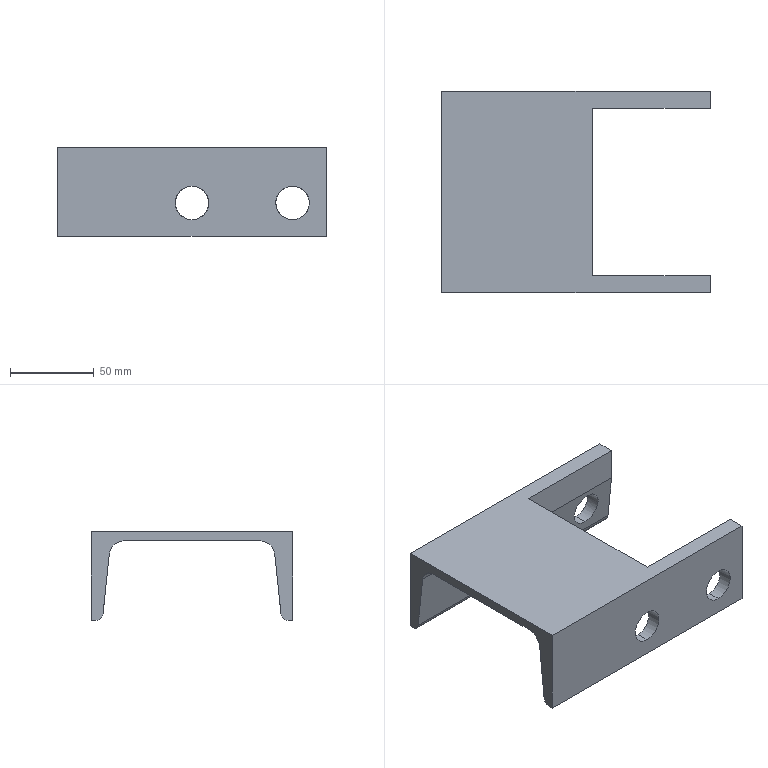Part | SolidWorks | features ICE 2, 3DProfileFeature 1, WeldMemberFeat 1, WeldmentFeature 1 | 1 solid | 26 faces | box 160 x 120 x 53 mm | volume 192954 mm3 | plane 14 | cylinder 12 | commonest cylinder face diameters 20 x8 9 x2 18 x2
STEP:
#1=CARTESIAN_POINT('',(80.,9.657,-23.));
#2=VERTEX_POINT('',#1);
#3=CARTESIAN_POINT('',(80.,7.555,-43.));
#4=VERTEX_POINT('',#3);
#5=CARTESIAN_POINT('',(80.,9.657,-23.));
#6=CARTESIAN_POINT('',(60.,9.657,-23.));
#7=CARTESIAN_POINT('',(60.,7.555,-43.));
#8=CARTESIAN_POINT('',(80.,7.555,-43.));
#9=(BOUNDED_CURVE()B_SPLINE_CURVE(3,(#5,#6,#7,#8),.UNSPECIFIED.,.F.,.F.)B_SPLINE_CURVE_WITH_KNOTS((4,4),(3.142,6.283),.UNSPECIFIED.)CURVE()GEOMETRIC_REPRESENTATION_ITEM()RATIONAL_B_SPLINE_CURVE((1.,0.3333,0.3333,1.))REPRESENTATION_ITEM(''));
#10=EDGE_CURVE('',#2,#4,#9,.T.);
#11=ORIENTED_EDGE('',*,*,#10,.F.);
#12=CARTESIAN_POINT('',(80.,0.,-23.));
#13=VERTEX_POINT('',#12);
#14=CARTESIAN_POINT('',(80.,148.284,-23.));
#15=DIRECTION('',(0.,-1.,0.));
#16=VECTOR('',#15,1000.);
#17=LINE('',#14,#16);
#18=EDGE_CURVE('',#2,#13,#17,.T.);
#19=ORIENTED_EDGE('',*,*,#18,.T.);
#20=CARTESIAN_POINT('',(80.,0.,-43.));
#21=VERTEX_POINT('',#20);
#22=CARTESIAN_POINT('',(80.,0.,-33.));
#23=DIRECTION('',(0.,-1.,0.));
#24=DIRECTION('',(0.,0.,-1.));
#25=AXIS2_PLACEMENT_3D('',#22,#23,#24);
#26=CIRCLE('',#25,10.);
#27=EDGE_CURVE('',#13,#21,#26,.T.);
#28=ORIENTED_EDGE('',*,*,#27,.T.);
#29=CARTESIAN_POINT('',(80.,148.284,-43.));
#30=DIRECTION('',(0.,-1.,0.));
#31=VECTOR('',#30,1000.);
#32=LINE('',#29,#31);
#33=EDGE_CURVE('',#4,#21,#32,.T.);
#34=ORIENTED_EDGE('',*,*,#33,.F.);
#35=EDGE_LOOP('',(#11,#19,#28,#34));
#36=FACE_OUTER_BOUND('',#35,.T.);
#37=CARTESIAN_POINT('',(80.,148.284,-33.));
#38=DIRECTION('',(0.,-1.,0.));
#39=DIRECTION('',(0.,0.,-1.));
#40=AXIS2_PLACEMENT_3D('',#37,#38,#39);
#41=CYLINDRICAL_SURFACE('',#40,10.);
#42=ADVANCED_FACE('',(#36),#41,.F.);
#43=CARTESIAN_POINT('',(80.,120.,-43.));
#44=VERTEX_POINT('',#43);
#45=CARTESIAN_POINT('',(80.,120.,-23.));
#46=VERTEX_POINT('',#45);
#47=CARTESIAN_POINT('',(80.,120.,-33.));
#48=DIRECTION('',(0.,1.,0.));
#49=DIRECTION('',(0.,0.,-1.));
#50=AXIS2_PLACEMENT_3D('',#47,#48,#49);
#51=CIRCLE('',#50,10.);
#52=EDGE_CURVE('',#44,#46,#51,.T.);
#53=ORIENTED_EDGE('',*,*,#52,.T.);
#54=CARTESIAN_POINT('',(80.,110.343,-23.));
#55=VERTEX_POINT('',#54);
#56=CARTESIAN_POINT('',(80.,148.284,-23.));
#57=DIRECTION('',(0.,-1.,0.));
#58=VECTOR('',#57,1000.);
#59=LINE('',#56,#58);
#60=EDGE_CURVE('',#46,#55,#59,.T.);
#61=ORIENTED_EDGE('',*,*,#60,.T.);
#62=CARTESIAN_POINT('',(80.,112.445,-43.));
#63=VERTEX_POINT('',#62);
#64=CARTESIAN_POINT('',(80.,112.445,-43.));
#65=CARTESIAN_POINT('',(60.,112.445,-43.));
#66=CARTESIAN_POINT('',(60.,110.343,-23.));
#67=CARTESIAN_POINT('',(80.,110.343,-23.));
#68=(BOUNDED_CURVE()B_SPLINE_CURVE(3,(#64,#65,#66,#67),.UNSPECIFIED.,.F.,.F.)B_SPLINE_CURVE_WITH_KNOTS((4,4),(3.142,6.283),.UNSPECIFIED.)CURVE()GEOMETRIC_REPRESENTATION_ITEM()RATIONAL_B_SPLINE_CURVE((1.,0.3333,0.3333,1.))REPRESENTATION_ITEM(''));
#69=EDGE_CURVE('',#63,#55,#68,.T.);
#70=ORIENTED_EDGE('',*,*,#69,.F.);
#71=CARTESIAN_POINT('',(80.,148.284,-43.));
#72=DIRECTION('',(0.,-1.,0.));
#73=VECTOR('',#72,1000.);
#74=LINE('',#71,#73);
#75=EDGE_CURVE('',#44,#63,#74,.T.);
#76=ORIENTED_EDGE('',*,*,#75,.F.);
#77=EDGE_LOOP('',(#53,#61,#70,#76));
#78=FACE_OUTER_BOUND('',#77,.T.);
#79=CARTESIAN_POINT('',(80.,148.284,-33.));
#80=DIRECTION('',(0.,-1.,0.));
#81=DIRECTION('',(0.,0.,-1.));
#82=AXIS2_PLACEMENT_3D('',#79,#80,#81);
#83=CYLINDRICAL_SURFACE('',#82,10.);
#84=ADVANCED_FACE('',(#78),#83,.F.);
#85=CARTESIAN_POINT('',(140.,9.657,-23.));
#86=VERTEX_POINT('',#85);
#87=CARTESIAN_POINT('',(140.,7.555,-43.));
#88=VERTEX_POINT('',#87);
#89=CARTESIAN_POINT('',(140.,9.657,-23.));
#90=CARTESIAN_POINT('',(120.,9.657,-23.));
#91=CARTESIAN_POINT('',(120.,7.555,-43.));
#92=CARTESIAN_POINT('',(140.,7.555,-43.));
#93=(BOUNDED_CURVE()B_SPLINE_CURVE(3,(#89,#90,#91,#92),.UNSPECIFIED.,.F.,.F.)B_SPLINE_CURVE_WITH_KNOTS((4,4),(3.142,6.283),.UNSPECIFIED.)CURVE()GEOMETRIC_REPRESENTATION_ITEM()RATIONAL_B_SPLINE_CURVE((1.,0.3333,0.3333,1.))REPRESENTATION_ITEM(''));
#94=EDGE_CURVE('',#86,#88,#93,.T.);
#95=ORIENTED_EDGE('',*,*,#94,.F.);
#96=CARTESIAN_POINT('',(140.,0.,-23.));
#97=VERTEX_POINT('',#96);
#98=CARTESIAN_POINT('',(140.,148.284,-23.));
#99=DIRECTION('',(0.,-1.,0.));
#100=VECTOR('',#99,1000.);
#101=LINE('',#98,#100);
#102=EDGE_CURVE('',#86,#97,#101,.T.);
#103=ORIENTED_EDGE('',*,*,#102,.T.);
#104=CARTESIAN_POINT('',(140.,0.,-43.));
#105=VERTEX_POINT('',#104);
#106=CARTESIAN_POINT('',(140.,0.,-33.));
#107=DIRECTION('',(0.,-1.,0.));
#108=DIRECTION('',(0.,0.,-1.));
#109=AXIS2_PLACEMENT_3D('',#106,#107,#108);
#110=CIRCLE('',#109,10.);
#111=EDGE_CURVE('',#97,#105,#110,.T.);
#112=ORIENTED_EDGE('',*,*,#111,.T.);
#113=CARTESIAN_POINT('',(140.,148.284,-43.));
#114=DIRECTION('',(0.,-1.,0.));
#115=VECTOR('',#114,1000.);
#116=LINE('',#113,#115);
#117=EDGE_CURVE('',#88,#105,#116,.T.);
#118=ORIENTED_EDGE('',*,*,#117,.F.);
#119=EDGE_LOOP('',(#95,#103,#112,#118));
#120=FACE_OUTER_BOUND('',#119,.T.);
#121=CARTESIAN_POINT('',(140.,148.284,-33.));
#122=DIRECTION('',(0.,-1.,0.));
#123=DIRECTION('',(0.,0.,-1.));
#124=AXIS2_PLACEMENT_3D('',#121,#122,#123);
#125=CYLINDRICAL_SURFACE('',#124,10.);
#126=ADVANCED_FACE('',(#120),#125,.F.);
#127=CARTESIAN_POINT('',(140.,120.,-43.));
#128=VERTEX_POINT('',#127);
#129=CARTESIAN_POINT('',(140.,120.,-23.));
#130=VERTEX_POINT('',#129);
#131=CARTESIAN_POINT('',(140.,120.,-33.));
#132=DIRECTION('',(0.,1.,0.));
#133=DIRECTION('',(0.,0.,-1.));
#134=AXIS2_PLACEMENT_3D('',#131,#132,#133);
#135=CIRCLE('',#134,10.);
#136=EDGE_CURVE('',#128,#130,#135,.T.);
#137=ORIENTED_EDGE('',*,*,#136,.T.);
#138=CARTESIAN_POINT('',(140.,110.343,-23.));
#139=VERTEX_POINT('',#138);
#140=CARTESIAN_POINT('',(140.,148.284,-23.));
#141=DIRECTION('',(0.,-1.,0.));
#142=VECTOR('',#141,1000.);
#143=LINE('',#140,#142);
#144=EDGE_CURVE('',#130,#139,#143,.T.);
#145=ORIENTED_EDGE('',*,*,#144,.T.);
#146=CARTESIAN_POINT('',(140.,112.445,-43.));
#147=VERTEX_POINT('',#146);
#148=CARTESIAN_POINT('',(140.,112.445,-43.));
#149=CARTESIAN_POINT('',(120.,112.445,-43.));
#150=CARTESIAN_POINT('',(120.,110.343,-23.));
#151=CARTESIAN_POINT('',(140.,110.343,-23.));
#152=(BOUNDED_CURVE()B_SPLINE_CURVE(3,(#148,#149,#150,#151),.UNSPECIFIED.,.F.,.F.)B_SPLINE_CURVE_WITH_KNOTS((4,4),(3.142,6.283),.UNSPECIFIED.)CURVE()GEOMETRIC_REPRESENTATION_ITEM()RATIONAL_B_SPLINE_CURVE((1.,0.3333,0.3333,1.))REPRESENTATION_ITEM(''));
#153=EDGE_CURVE('',#147,#139,#152,.T.);
#154=ORIENTED_EDGE('',*,*,#153,.F.);
#155=CARTESIAN_POINT('',(140.,148.284,-43.));
#156=DIRECTION('',(0.,-1.,0.));
#157=VECTOR('',#156,1000.);
#158=LINE('',#155,#157);
#159=EDGE_CURVE('',#128,#147,#158,.T.);
#160=ORIENTED_EDGE('',*,*,#159,.F.);
#161=EDGE_LOOP('',(#137,#145,#154,#160));
#162=FACE_OUTER_BOUND('',#161,.T.);
#163=CARTESIAN_POINT('',(140.,148.284,-33.));
#164=DIRECTION('',(0.,-1.,0.));
#165=DIRECTION('',(0.,0.,-1.));
#166=AXIS2_PLACEMENT_3D('',#163,#164,#165);
#167=CYLINDRICAL_SURFACE('',#166,10.);
#168=ADVANCED_FACE('',(#162),#167,.F.);
#169=CARTESIAN_POINT('',(160.,110.,-19.736));
#170=VERTEX_POINT('',#169);
#171=CARTESIAN_POINT('',(160.,110.,0.));
#172=VERTEX_POINT('',#171);
#173=CARTESIAN_POINT('',(160.,110.,-48.5));
#174=DIRECTION('',(0.,0.,1.));
#175=VECTOR('',#174,1000.);
#176=LINE('',#173,#175);
#177=EDGE_CURVE('',#170,#172,#176,.T.);
#178=ORIENTED_EDGE('',*,*,#177,.F.);
#179=CARTESIAN_POINT('',(160.,113.073,-48.97));
#180=VERTEX_POINT('',#179);
#181=CARTESIAN_POINT('',(160.,109.351,-13.559));
#182=DIRECTION('',(0.,0.1045,-0.9945));
#183=VECTOR('',#182,1000.);
#184=LINE('',#181,#183);
#185=EDGE_CURVE('',#170,#180,#184,.T.);
#186=ORIENTED_EDGE('',*,*,#185,.T.);
#187=CARTESIAN_POINT('',(160.,117.548,-53.));
#188=VERTEX_POINT('',#187);
#189=CARTESIAN_POINT('',(160.,117.548,-48.5));
#190=DIRECTION('',(1.,0.,0.));
#191=DIRECTION('',(0.,0.,-1.));
#192=AXIS2_PLACEMENT_3D('',#189,#190,#191);
#193=CIRCLE('',#192,4.5);
#194=EDGE_CURVE('',#180,#188,#193,.T.);
#195=ORIENTED_EDGE('',*,*,#194,.T.);
#196=CARTESIAN_POINT('',(160.,120.,-53.));
#197=VERTEX_POINT('',#196);
#198=CARTESIAN_POINT('',(160.,120.,-53.));
#199=DIRECTION('',(0.,1.,0.));
#200=VECTOR('',#199,1000.);
#201=LINE('',#198,#200);
#202=EDGE_CURVE('',#188,#197,#201,.T.);
#203=ORIENTED_EDGE('',*,*,#202,.T.);
#204=CARTESIAN_POINT('',(160.,120.,0.));
#205=VERTEX_POINT('',#204);
#206=CARTESIAN_POINT('',(160.,120.,-53.));
#207=DIRECTION('',(0.,0.,1.));
#208=VECTOR('',#207,1000.);
#209=LINE('',#206,#208);
#210=EDGE_CURVE('',#197,#205,#209,.T.);
#211=ORIENTED_EDGE('',*,*,#210,.T.);
#212=CARTESIAN_POINT('',(160.,120.,0.));
#213=DIRECTION('',(0.,-1.,0.));
#214=VECTOR('',#213,1000.);
#215=LINE('',#212,#214);
#216=EDGE_CURVE('',#205,#172,#215,.T.);
#217=ORIENTED_EDGE('',*,*,#216,.T.);
#218=EDGE_LOOP('',(#178,#186,#195,#203,#211,#217));
#219=FACE_OUTER_BOUND('',#218,.T.);
#220=CARTESIAN_POINT('',(160.,117.548,-48.5));
#221=DIRECTION('',(1.,0.,0.));
#222=DIRECTION('',(0.,0.,-1.));
#223=AXIS2_PLACEMENT_3D('',#220,#221,#222);
#224=PLANE('',#223);
#225=ADVANCED_FACE('',(#219),#224,.T.);
#226=CARTESIAN_POINT('',(0.,113.073,-48.97));
#227=VERTEX_POINT('',#226);
#228=CARTESIAN_POINT('',(0.,117.548,-53.));
#229=VERTEX_POINT('',#228);
#230=CARTESIAN_POINT('',(0.,117.548,-48.5));
#231=DIRECTION('',(1.,0.,0.));
#232=DIRECTION('',(0.,0.,-1.));
#233=AXIS2_PLACEMENT_3D('',#230,#231,#232);
#234=CIRCLE('',#233,4.5);
#235=EDGE_CURVE('',#227,#229,#234,.T.);
#236=ORIENTED_EDGE('',*,*,#235,.T.);
#237=CARTESIAN_POINT('',(160.,117.548,-53.));
#238=DIRECTION('',(-1.,0.,0.));
#239=VECTOR('',#238,1000.);
#240=LINE('',#237,#239);
#241=EDGE_CURVE('',#188,#229,#240,.T.);
#242=ORIENTED_EDGE('',*,*,#241,.F.);
#243=ORIENTED_EDGE('',*,*,#194,.F.);
#244=CARTESIAN_POINT('',(160.,113.073,-48.97));
#245=DIRECTION('',(-1.,0.,0.));
#246=VECTOR('',#245,1000.);
#247=LINE('',#244,#246);
#248=EDGE_CURVE('',#180,#227,#247,.T.);
#249=ORIENTED_EDGE('',*,*,#248,.T.);
#250=EDGE_LOOP('',(#236,#242,#243,#249));
#251=FACE_OUTER_BOUND('',#250,.T.);
#252=CARTESIAN_POINT('',(160.,117.548,-48.5));
#253=DIRECTION('',(-1.,0.,0.));
#254=DIRECTION('',(0.,0.,1.));
#255=AXIS2_PLACEMENT_3D('',#252,#253,#254);
#256=CYLINDRICAL_SURFACE('',#255,4.5);
#257=ADVANCED_FACE('',(#251),#256,.T.);
#258=CARTESIAN_POINT('',(0.,120.,-53.));
#259=VERTEX_POINT('',#258);
#260=CARTESIAN_POINT('',(0.,120.,-53.));
#261=DIRECTION('',(0.,1.,0.));
#262=VECTOR('',#261,1000.);
#263=LINE('',#260,#262);
#264=EDGE_CURVE('',#229,#259,#263,.T.);
#265=ORIENTED_EDGE('',*,*,#264,.T.);
#266=CARTESIAN_POINT('',(160.,120.,-53.));
#267=DIRECTION('',(-1.,0.,0.));
#268=VECTOR('',#267,1000.);
#269=LINE('',#266,#268);
#270=EDGE_CURVE('',#197,#259,#269,.T.);
#271=ORIENTED_EDGE('',*,*,#270,.F.);
#272=ORIENTED_EDGE('',*,*,#202,.F.);
#273=ORIENTED_EDGE('',*,*,#241,.T.);
#274=EDGE_LOOP('',(#265,#271,#272,#273));
#275=FACE_OUTER_BOUND('',#274,.T.);
#276=CARTESIAN_POINT('',(160.,120.,-53.));
#277=DIRECTION('',(0.,0.,1.));
#278=DIRECTION('',(0.,-1.,0.));
#279=AXIS2_PLACEMENT_3D('',#276,#277,#278);
#280=PLANE('',#279);
#281=ADVANCED_FACE('',(#275),#280,.F.);
#282=ORIENTED_EDGE('',*,*,#52,.F.);
#283=CARTESIAN_POINT('',(80.,120.,-33.));
#284=DIRECTION('',(0.,1.,0.));
#285=DIRECTION('',(0.,0.,-1.));
#286=AXIS2_PLACEMENT_3D('',#283,#284,#285);
#287=CIRCLE('',#286,10.);
#288=EDGE_CURVE('',#46,#44,#287,.T.);
#289=ORIENTED_EDGE('',*,*,#288,.F.);
#290=EDGE_LOOP('',(#282,#289));
#291=FACE_BOUND('',#290,.T.);
#292=ORIENTED_EDGE('',*,*,#136,.F.);
#293=CARTESIAN_POINT('',(140.,120.,-33.));
#294=DIRECTION('',(0.,1.,0.));
#295=DIRECTION('',(0.,0.,-1.));
#296=AXIS2_PLACEMENT_3D('',#293,#294,#295);
#297=CIRCLE('',#296,10.);
#298=EDGE_CURVE('',#130,#128,#297,.T.);
#299=ORIENTED_EDGE('',*,*,#298,.F.);
#300=EDGE_LOOP('',(#292,#299));
#301=FACE_BOUND('',#300,.T.);
#302=CARTESIAN_POINT('',(0.,120.,0.));
#303=VERTEX_POINT('',#302);
#304=CARTESIAN_POINT('',(0.,120.,-53.));
#305=DIRECTION('',(0.,0.,1.));
#306=VECTOR('',#305,1000.);
#307=LINE('',#304,#306);
#308=EDGE_CURVE('',#259,#303,#307,.T.);
#309=ORIENTED_EDGE('',*,*,#308,.T.);
#310=CARTESIAN_POINT('',(160.,120.,0.));
#311=DIRECTION('',(-1.,0.,0.));
#312=VECTOR('',#311,1000.);
#313=LINE('',#310,#312);
#314=EDGE_CURVE('',#205,#303,#313,.T.);
#315=ORIENTED_EDGE('',*,*,#314,.F.);
#316=ORIENTED_EDGE('',*,*,#210,.F.);
#317=ORIENTED_EDGE('',*,*,#270,.T.);
#318=EDGE_LOOP('',(#309,#315,#316,#317));
#319=FACE_OUTER_BOUND('',#318,.T.);
#320=CARTESIAN_POINT('',(160.,120.,-53.));
#321=DIRECTION('',(0.,-1.,0.));
#322=DIRECTION('',(0.,0.,-1.));
#323=AXIS2_PLACEMENT_3D('',#320,#321,#322);
#324=PLANE('',#323);
#325=ADVANCED_FACE('',(#291,#301,#319),#324,.F.);
#326=CARTESIAN_POINT('',(90.,110.,0.));
#327=VERTEX_POINT('',#326);
#328=CARTESIAN_POINT('',(90.,10.,0.));
#329=VERTEX_POINT('',#328);
#330=CARTESIAN_POINT('',(90.,110.,0.));
#331=DIRECTION('',(0.,-1.,0.));
#332=VECTOR('',#331,1000.);
#333=LINE('',#330,#332);
#334=EDGE_CURVE('',#327,#329,#333,.T.);
#335=ORIENTED_EDGE('',*,*,#334,.F.);
#336=CARTESIAN_POINT('',(90.,110.,0.));
#337=DIRECTION('',(-1.,0.,0.));
#338=VECTOR('',#337,1000.);
#339=LINE('',#336,#338);
#340=EDGE_CURVE('',#172,#327,#339,.T.);
#341=ORIENTED_EDGE('',*,*,#340,.F.);
#342=ORIENTED_EDGE('',*,*,#216,.F.);
#343=ORIENTED_EDGE('',*,*,#314,.T.);
#344=CARTESIAN_POINT('',(0.,0.,0.));
#345=VERTEX_POINT('',#344);
#346=CARTESIAN_POINT('',(0.,120.,0.));
#347=DIRECTION('',(0.,-1.,0.));
#348=VECTOR('',#347,1000.);
#349=LINE('',#346,#348);
#350=EDGE_CURVE('',#303,#345,#349,.T.);
#351=ORIENTED_EDGE('',*,*,#350,.T.);
#352=CARTESIAN_POINT('',(160.,0.,0.));
#353=VERTEX_POINT('',#352);
#354=CARTESIAN_POINT('',(160.,0.,0.));
#355=DIRECTION('',(-1.,0.,0.));
#356=VECTOR('',#355,1000.);
#357=LINE('',#354,#356);
#358=EDGE_CURVE('',#353,#345,#357,.T.);
#359=ORIENTED_EDGE('',*,*,#358,.F.);
#360=CARTESIAN_POINT('',(160.,10.,0.));
#361=VERTEX_POINT('',#360);
#362=CARTESIAN_POINT('',(160.,120.,0.));
#363=DIRECTION('',(0.,-1.,0.));
#364=VECTOR('',#363,1000.);
#365=LINE('',#362,#364);
#366=EDGE_CURVE('',#361,#353,#365,.T.);
#367=ORIENTED_EDGE('',*,*,#366,.F.);
#368=CARTESIAN_POINT('',(90.,10.,0.));
#369=DIRECTION('',(1.,0.,0.));
#370=VECTOR('',#369,1000.);
#371=LINE('',#368,#370);
#372=EDGE_CURVE('',#329,#361,#371,.T.);
#373=ORIENTED_EDGE('',*,*,#372,.F.);
#374=EDGE_LOOP('',(#335,#341,#342,#343,#351,#359,#367,#373));
#375=FACE_OUTER_BOUND('',#374,.T.);
#376=CARTESIAN_POINT('',(160.,120.,0.));
#377=DIRECTION('',(0.,0.,-1.));
#378=DIRECTION('',(-1.,0.,0.));
#379=AXIS2_PLACEMENT_3D('',#376,#377,#378);
#380=PLANE('',#379);
#381=ADVANCED_FACE('',(#375),#380,.F.);
#382=CARTESIAN_POINT('',(80.,0.,-33.));
#383=DIRECTION('',(0.,-1.,0.));
#384=DIRECTION('',(0.,0.,-1.));
#385=AXIS2_PLACEMENT_3D('',#382,#383,#384);
#386=CIRCLE('',#385,10.);
#387=EDGE_CURVE('',#21,#13,#386,.T.);
#388=ORIENTED_EDGE('',*,*,#387,.F.);
#389=ORIENTED_EDGE('',*,*,#27,.F.);
#390=EDGE_LOOP('',(#388,#389));
#391=FACE_BOUND('',#390,.T.);
#392=CARTESIAN_POINT('',(140.,0.,-33.));
#393=DIRECTION('',(0.,-1.,0.));
#394=DIRECTION('',(0.,0.,-1.));
#395=AXIS2_PLACEMENT_3D('',#392,#393,#394);
#396=CIRCLE('',#395,10.);
#397=EDGE_CURVE('',#105,#97,#396,.T.);
#398=ORIENTED_EDGE('',*,*,#397,.F.);
#399=ORIENTED_EDGE('',*,*,#111,.F.);
#400=EDGE_LOOP('',(#398,#399));
#401=FACE_BOUND('',#400,.T.);
#402=CARTESIAN_POINT('',(0.,0.,-53.));
#403=VERTEX_POINT('',#402);
#404=CARTESIAN_POINT('',(0.,0.,-53.));
#405=DIRECTION('',(0.,0.,-1.));
#406=VECTOR('',#405,1000.);
#407=LINE('',#404,#406);
#408=EDGE_CURVE('',#345,#403,#407,.T.);
#409=ORIENTED_EDGE('',*,*,#408,.T.);
#410=CARTESIAN_POINT('',(160.,0.,-53.));
#411=VERTEX_POINT('',#410);
#412=CARTESIAN_POINT('',(160.,0.,-53.));
#413=DIRECTION('',(-1.,0.,0.));
#414=VECTOR('',#413,1000.);
#415=LINE('',#412,#414);
#416=EDGE_CURVE('',#411,#403,#415,.T.);
#417=ORIENTED_EDGE('',*,*,#416,.F.);
#418=CARTESIAN_POINT('',(160.,0.,-53.));
#419=DIRECTION('',(0.,0.,-1.));
#420=VECTOR('',#419,1000.);
#421=LINE('',#418,#420);
#422=EDGE_CURVE('',#353,#411,#421,.T.);
#423=ORIENTED_EDGE('',*,*,#422,.F.);
#424=ORIENTED_EDGE('',*,*,#358,.T.);
#425=EDGE_LOOP('',(#409,#417,#423,#424));
#426=FACE_OUTER_BOUND('',#425,.T.);
#427=CARTESIAN_POINT('',(160.,0.,-53.));
#428=DIRECTION('',(0.,1.,0.));
#429=DIRECTION('',(0.,0.,1.));
#430=AXIS2_PLACEMENT_3D('',#427,#428,#429);
#431=PLANE('',#430);
#432=ADVANCED_FACE('',(#391,#401,#426),#431,.F.);
#433=CARTESIAN_POINT('',(0.,2.452,-53.));
#434=VERTEX_POINT('',#433);
#435=CARTESIAN_POINT('',(0.,0.,-53.));
#436=DIRECTION('',(0.,1.,0.));
#437=VECTOR('',#436,1000.);
#438=LINE('',#435,#437);
#439=EDGE_CURVE('',#403,#434,#438,.T.);
#440=ORIENTED_EDGE('',*,*,#439,.T.);
#441=CARTESIAN_POINT('',(160.,2.452,-53.));
#442=VERTEX_POINT('',#441);
#443=CARTESIAN_POINT('',(160.,2.452,-53.));
#444=DIRECTION('',(-1.,0.,0.));
#445=VECTOR('',#444,1000.);
#446=LINE('',#443,#445);
#447=EDGE_CURVE('',#442,#434,#446,.T.);
#448=ORIENTED_EDGE('',*,*,#447,.F.);
#449=CARTESIAN_POINT('',(160.,0.,-53.));
#450=DIRECTION('',(0.,1.,0.));
#451=VECTOR('',#450,1000.);
#452=LINE('',#449,#451);
#453=EDGE_CURVE('',#411,#442,#452,.T.);
#454=ORIENTED_EDGE('',*,*,#453,.F.);
#455=ORIENTED_EDGE('',*,*,#416,.T.);
#456=EDGE_LOOP('',(#440,#448,#454,#455));
#457=FACE_OUTER_BOUND('',#456,.T.);
#458=CARTESIAN_POINT('',(160.,0.,-53.));
#459=DIRECTION('',(0.,0.,1.));
#460=DIRECTION('',(0.,-1.,0.));
#461=AXIS2_PLACEMENT_3D('',#458,#459,#460);
#462=PLANE('',#461);
#463=ADVANCED_FACE('',(#457),#462,.F.);
#464=CARTESIAN_POINT('',(0.,6.927,-48.97));
#465=VERTEX_POINT('',#464);
#466=CARTESIAN_POINT('',(0.,2.452,-48.5));
#467=DIRECTION('',(1.,0.,0.));
#468=DIRECTION('',(0.,0.,1.));
#469=AXIS2_PLACEMENT_3D('',#466,#467,#468);
#470=CIRCLE('',#469,4.5);
#471=EDGE_CURVE('',#434,#465,#470,.T.);
#472=ORIENTED_EDGE('',*,*,#471,.T.);
#473=CARTESIAN_POINT('',(160.,6.927,-48.97));
#474=VERTEX_POINT('',#473);
#475=CARTESIAN_POINT('',(160.,6.927,-48.97));
#476=DIRECTION('',(-1.,0.,0.));
#477=VECTOR('',#476,1000.);
#478=LINE('',#475,#477);
#479=EDGE_CURVE('',#474,#465,#478,.T.);
#480=ORIENTED_EDGE('',*,*,#479,.F.);
#481=CARTESIAN_POINT('',(160.,2.452,-48.5));
#482=DIRECTION('',(1.,0.,0.));
#483=DIRECTION('',(0.,0.,1.));
#484=AXIS2_PLACEMENT_3D('',#481,#482,#483);
#485=CIRCLE('',#484,4.5);
#486=EDGE_CURVE('',#442,#474,#485,.T.);
#487=ORIENTED_EDGE('',*,*,#486,.F.);
#488=ORIENTED_EDGE('',*,*,#447,.T.);
#489=EDGE_LOOP('',(#472,#480,#487,#488));
#490=FACE_OUTER_BOUND('',#489,.T.);
#491=CARTESIAN_POINT('',(160.,2.452,-48.5));
#492=DIRECTION('',(-1.,0.,0.));
#493=DIRECTION('',(0.,0.,1.));
#494=AXIS2_PLACEMENT_3D('',#491,#492,#493);
#495=CYLINDRICAL_SURFACE('',#494,4.5);
#496=ADVANCED_FACE('',(#490),#495,.T.);
#497=CARTESIAN_POINT('',(80.,7.555,-43.));
#498=CARTESIAN_POINT('',(100.,7.555,-43.));
#499=CARTESIAN_POINT('',(100.,9.657,-23.));
#500=CARTESIAN_POINT('',(80.,9.657,-23.));
#501=(BOUNDED_CURVE()B_SPLINE_CURVE(3,(#497,#498,#499,#500),.UNSPECIFIED.,.F.,.F.)B_SPLINE_CURVE_WITH_KNOTS((4,4),(0.,3.142),.UNSPECIFIED.)CURVE()GEOMETRIC_REPRESENTATION_ITEM()RATIONAL_B_SPLINE_CURVE((1.,0.3333,0.3333,1.))REPRESENTATION_ITEM(''));
#502=EDGE_CURVE('',#4,#2,#501,.T.);
#503=ORIENTED_EDGE('',*,*,#502,.T.);
#504=ORIENTED_EDGE('',*,*,#10,.T.);
#505=EDGE_LOOP('',(#503,#504));
#506=FACE_BOUND('',#505,.T.);
#507=CARTESIAN_POINT('',(140.,7.555,-43.));
#508=CARTESIAN_POINT('',(160.,7.555,-43.));
#509=CARTESIAN_POINT('',(160.,9.657,-23.));
#510=CARTESIAN_POINT('',(140.,9.657,-23.));
#511=(BOUNDED_CURVE()B_SPLINE_CURVE(3,(#507,#508,#509,#510),.UNSPECIFIED.,.F.,.F.)B_SPLINE_CURVE_WITH_KNOTS((4,4),(0.,3.142),.UNSPECIFIED.)CURVE()GEOMETRIC_REPRESENTATION_ITEM()RATIONAL_B_SPLINE_CURVE((1.,0.3333,0.3333,1.))REPRESENTATION_ITEM(''));
#512=EDGE_CURVE('',#88,#86,#511,.T.);
#513=ORIENTED_EDGE('',*,*,#512,.T.);
#514=ORIENTED_EDGE('',*,*,#94,.T.);
#515=EDGE_LOOP('',(#513,#514));
#516=FACE_BOUND('',#515,.T.);
#517=CARTESIAN_POINT('',(90.,10.649,-13.559));
#518=VERTEX_POINT('',#517);
#519=CARTESIAN_POINT('',(0.,10.649,-13.559));
#520=VERTEX_POINT('',#519);
#521=CARTESIAN_POINT('',(160.,10.649,-13.559));
#522=DIRECTION('',(-1.,0.,0.));
#523=VECTOR('',#522,1000.);
#524=LINE('',#521,#523);
#525=EDGE_CURVE('',#518,#520,#524,.T.);
#526=ORIENTED_EDGE('',*,*,#525,.F.);
#527=CARTESIAN_POINT('',(90.,10.,-19.736));
#528=VERTEX_POINT('',#527);
#529=CARTESIAN_POINT('',(90.,10.649,-13.559));
#530=DIRECTION('',(0.,-0.1045,-0.9945));
#531=VECTOR('',#530,1000.);
#532=LINE('',#529,#531);
#533=EDGE_CURVE('',#518,#528,#532,.T.);
#534=ORIENTED_EDGE('',*,*,#533,.T.);
#535=CARTESIAN_POINT('',(160.,10.,-19.736));
#536=VERTEX_POINT('',#535);
#537=CARTESIAN_POINT('',(160.,10.,-19.736));
#538=DIRECTION('',(1.,0.,0.));
#539=VECTOR('',#538,1000.);
#540=LINE('',#537,#539);
#541=EDGE_CURVE('',#528,#536,#540,.T.);
#542=ORIENTED_EDGE('',*,*,#541,.T.);
#543=CARTESIAN_POINT('',(160.,10.649,-13.559));
#544=DIRECTION('',(0.,0.1045,0.9945));
#545=VECTOR('',#544,1000.);
#546=LINE('',#543,#545);
#547=EDGE_CURVE('',#474,#536,#546,.T.);
#548=ORIENTED_EDGE('',*,*,#547,.F.);
#549=ORIENTED_EDGE('',*,*,#479,.T.);
#550=CARTESIAN_POINT('',(0.,10.649,-13.559));
#551=DIRECTION('',(0.,0.1045,0.9945));
#552=VECTOR('',#551,1000.);
#553=LINE('',#550,#552);
#554=EDGE_CURVE('',#465,#520,#553,.T.);
#555=ORIENTED_EDGE('',*,*,#554,.T.);
#556=EDGE_LOOP('',(#526,#534,#542,#548,#549,#555));
#557=FACE_OUTER_BOUND('',#556,.T.);
#558=CARTESIAN_POINT('',(160.,10.649,-13.559));
#559=DIRECTION('',(0.,-0.9945,0.1045));
#560=DIRECTION('',(0.,-0.1045,-0.9945));
#561=AXIS2_PLACEMENT_3D('',#558,#559,#560);
#562=PLANE('',#561);
#563=ADVANCED_FACE('',(#506,#516,#557),#562,.F.);
#564=CARTESIAN_POINT('',(90.,19.6,-5.5));
#565=VERTEX_POINT('',#564);
#566=CARTESIAN_POINT('',(0.,19.6,-5.5));
#567=VERTEX_POINT('',#566);
#568=CARTESIAN_POINT('',(160.,19.6,-5.5));
#569=DIRECTION('',(-1.,0.,0.));
#570=VECTOR('',#569,1000.);
#571=LINE('',#568,#570);
#572=EDGE_CURVE('',#565,#567,#571,.T.);
#573=ORIENTED_EDGE('',*,*,#572,.F.);
#574=CARTESIAN_POINT('',(90.,19.6,-14.5));
#575=DIRECTION('',(1.,0.,0.));
#576=DIRECTION('',(0.,-1.,0.));
#577=AXIS2_PLACEMENT_3D('',#574,#575,#576);
#578=CIRCLE('',#577,9.);
#579=EDGE_CURVE('',#565,#518,#578,.T.);
#580=ORIENTED_EDGE('',*,*,#579,.T.);
#581=ORIENTED_EDGE('',*,*,#525,.T.);
#582=CARTESIAN_POINT('',(0.,19.6,-14.5));
#583=DIRECTION('',(-1.,0.,0.));
#584=DIRECTION('',(0.,0.,-1.));
#585=AXIS2_PLACEMENT_3D('',#582,#583,#584);
#586=CIRCLE('',#585,9.);
#587=EDGE_CURVE('',#520,#567,#586,.T.);
#588=ORIENTED_EDGE('',*,*,#587,.T.);
#589=EDGE_LOOP('',(#573,#580,#581,#588));
#590=FACE_OUTER_BOUND('',#589,.T.);
#591=CARTESIAN_POINT('',(160.,19.6,-14.5));
#592=DIRECTION('',(-1.,0.,0.));
#593=DIRECTION('',(0.,0.,1.));
#594=AXIS2_PLACEMENT_3D('',#591,#592,#593);
#595=CYLINDRICAL_SURFACE('',#594,9.);
#596=ADVANCED_FACE('',(#590),#595,.F.);
#597=CARTESIAN_POINT('',(90.,100.4,-5.5));
#598=VERTEX_POINT('',#597);
#599=CARTESIAN_POINT('',(0.,100.4,-5.5));
#600=VERTEX_POINT('',#599);
#601=CARTESIAN_POINT('',(160.,100.4,-5.5));
#602=DIRECTION('',(-1.,0.,0.));
#603=VECTOR('',#602,1000.);
#604=LINE('',#601,#603);
#605=EDGE_CURVE('',#598,#600,#604,.T.);
#606=ORIENTED_EDGE('',*,*,#605,.F.);
#607=CARTESIAN_POINT('',(90.,100.4,-5.5));
#608=DIRECTION('',(0.,-1.,0.));
#609=VECTOR('',#608,1000.);
#610=LINE('',#607,#609);
#611=EDGE_CURVE('',#598,#565,#610,.T.);
#612=ORIENTED_EDGE('',*,*,#611,.T.);
#613=ORIENTED_EDGE('',*,*,#572,.T.);
#614=CARTESIAN_POINT('',(0.,100.4,-5.5));
#615=DIRECTION('',(0.,1.,0.));
#616=VECTOR('',#615,1000.);
#617=LINE('',#614,#616);
#618=EDGE_CURVE('',#567,#600,#617,.T.);
#619=ORIENTED_EDGE('',*,*,#618,.T.);
#620=EDGE_LOOP('',(#606,#612,#613,#619));
#621=FACE_OUTER_BOUND('',#620,.T.);
#622=CARTESIAN_POINT('',(160.,100.4,-5.5));
#623=DIRECTION('',(0.,0.,1.));
#624=DIRECTION('',(1.,0.,0.));
#625=AXIS2_PLACEMENT_3D('',#622,#623,#624);
#626=PLANE('',#625);
#627=ADVANCED_FACE('',(#621),#626,.F.);
#628=CARTESIAN_POINT('',(90.,109.351,-13.559));
#629=VERTEX_POINT('',#628);
#630=CARTESIAN_POINT('',(0.,109.351,-13.559));
#631=VERTEX_POINT('',#630);
#632=CARTESIAN_POINT('',(160.,109.351,-13.559));
#633=DIRECTION('',(-1.,0.,0.));
#634=VECTOR('',#633,1000.);
#635=LINE('',#632,#634);
#636=EDGE_CURVE('',#629,#631,#635,.T.);
#637=ORIENTED_EDGE('',*,*,#636,.F.);
#638=CARTESIAN_POINT('',(90.,100.4,-14.5));
#639=DIRECTION('',(1.,0.,0.));
#640=DIRECTION('',(0.,-1.,0.));
#641=AXIS2_PLACEMENT_3D('',#638,#639,#640);
#642=CIRCLE('',#641,9.);
#643=EDGE_CURVE('',#629,#598,#642,.T.);
#644=ORIENTED_EDGE('',*,*,#643,.T.);
#645=ORIENTED_EDGE('',*,*,#605,.T.);
#646=CARTESIAN_POINT('',(0.,100.4,-14.5));
#647=DIRECTION('',(-1.,0.,0.));
#648=DIRECTION('',(0.,0.,1.));
#649=AXIS2_PLACEMENT_3D('',#646,#647,#648);
#650=CIRCLE('',#649,9.);
#651=EDGE_CURVE('',#600,#631,#650,.T.);
#652=ORIENTED_EDGE('',*,*,#651,.T.);
#653=EDGE_LOOP('',(#637,#644,#645,#652));
#654=FACE_OUTER_BOUND('',#653,.T.);
#655=CARTESIAN_POINT('',(160.,100.4,-14.5));
#656=DIRECTION('',(-1.,0.,0.));
#657=DIRECTION('',(0.,0.,1.));
#658=AXIS2_PLACEMENT_3D('',#655,#656,#657);
#659=CYLINDRICAL_SURFACE('',#658,9.);
#660=ADVANCED_FACE('',(#654),#659,.F.);
#661=ORIENTED_EDGE('',*,*,#69,.T.);
#662=CARTESIAN_POINT('',(80.,110.343,-23.));
#663=CARTESIAN_POINT('',(100.,110.343,-23.));
#664=CARTESIAN_POINT('',(100.,112.445,-43.));
#665=CARTESIAN_POINT('',(80.,112.445,-43.));
#666=(BOUNDED_CURVE()B_SPLINE_CURVE(3,(#662,#663,#664,#665),.UNSPECIFIED.,.F.,.F.)B_SPLINE_CURVE_WITH_KNOTS((4,4),(0.,3.142),.UNSPECIFIED.)CURVE()GEOMETRIC_REPRESENTATION_ITEM()RATIONAL_B_SPLINE_CURVE((1.,0.3333,0.3333,1.))REPRESENTATION_ITEM(''));
#667=EDGE_CURVE('',#55,#63,#666,.T.);
#668=ORIENTED_EDGE('',*,*,#667,.T.);
#669=EDGE_LOOP('',(#661,#668));
#670=FACE_BOUND('',#669,.T.);
#671=ORIENTED_EDGE('',*,*,#153,.T.);
#672=CARTESIAN_POINT('',(140.,110.343,-23.));
#673=CARTESIAN_POINT('',(160.,110.343,-23.));
#674=CARTESIAN_POINT('',(160.,112.445,-43.));
#675=CARTESIAN_POINT('',(140.,112.445,-43.));
#676=(BOUNDED_CURVE()B_SPLINE_CURVE(3,(#672,#673,#674,#675),.UNSPECIFIED.,.F.,.F.)B_SPLINE_CURVE_WITH_KNOTS((4,4),(0.,3.142),.UNSPECIFIED.)CURVE()GEOMETRIC_REPRESENTATION_ITEM()RATIONAL_B_SPLINE_CURVE((1.,0.3333,0.3333,1.))REPRESENTATION_ITEM(''));
#677=EDGE_CURVE('',#139,#147,#676,.T.);
#678=ORIENTED_EDGE('',*,*,#677,.T.);
#679=EDGE_LOOP('',(#671,#678));
#680=FACE_BOUND('',#679,.T.);
#681=CARTESIAN_POINT('',(90.,110.,-19.736));
#682=VERTEX_POINT('',#681);
#683=CARTESIAN_POINT('',(160.,110.,-19.736));
#684=DIRECTION('',(-1.,0.,0.));
#685=VECTOR('',#684,1000.);
#686=LINE('',#683,#685);
#687=EDGE_CURVE('',#170,#682,#686,.T.);
#688=ORIENTED_EDGE('',*,*,#687,.T.);
#689=CARTESIAN_POINT('',(90.,109.351,-13.559));
#690=DIRECTION('',(0.,-0.1045,0.9945));
#691=VECTOR('',#690,1000.);
#692=LINE('',#689,#691);
#693=EDGE_CURVE('',#682,#629,#692,.T.);
#694=ORIENTED_EDGE('',*,*,#693,.T.);
#695=ORIENTED_EDGE('',*,*,#636,.T.);
#696=CARTESIAN_POINT('',(0.,109.351,-13.559));
#697=DIRECTION('',(0.,0.1045,-0.9945));
#698=VECTOR('',#697,1000.);
#699=LINE('',#696,#698);
#700=EDGE_CURVE('',#631,#227,#699,.T.);
#701=ORIENTED_EDGE('',*,*,#700,.T.);
#702=ORIENTED_EDGE('',*,*,#248,.F.);
#703=ORIENTED_EDGE('',*,*,#185,.F.);
#704=EDGE_LOOP('',(#688,#694,#695,#701,#702,#703));
#705=FACE_OUTER_BOUND('',#704,.T.);
#706=CARTESIAN_POINT('',(160.,109.351,-13.559));
#707=DIRECTION('',(0.,0.9945,0.1045));
#708=DIRECTION('',(0.,-0.1045,0.9945));
#709=AXIS2_PLACEMENT_3D('',#706,#707,#708);
#710=PLANE('',#709);
#711=ADVANCED_FACE('',(#670,#680,#705),#710,.F.);
#712=CARTESIAN_POINT('',(160.,10.,-48.5));
#713=DIRECTION('',(0.,0.,-1.));
#714=VECTOR('',#713,1000.);
#715=LINE('',#712,#714);
#716=EDGE_CURVE('',#361,#536,#715,.T.);
#717=ORIENTED_EDGE('',*,*,#716,.F.);
#718=ORIENTED_EDGE('',*,*,#366,.T.);
#719=ORIENTED_EDGE('',*,*,#422,.T.);
#720=ORIENTED_EDGE('',*,*,#453,.T.);
#721=ORIENTED_EDGE('',*,*,#486,.T.);
#722=ORIENTED_EDGE('',*,*,#547,.T.);
#723=EDGE_LOOP('',(#717,#718,#719,#720,#721,#722));
#724=FACE_OUTER_BOUND('',#723,.T.);
#725=CARTESIAN_POINT('',(160.,117.548,-48.5));
#726=DIRECTION('',(1.,0.,0.));
#727=DIRECTION('',(0.,0.,-1.));
#728=AXIS2_PLACEMENT_3D('',#725,#726,#727);
#729=PLANE('',#728);
#730=ADVANCED_FACE('',(#724),#729,.T.);
#731=ORIENTED_EDGE('',*,*,#235,.F.);
#732=ORIENTED_EDGE('',*,*,#700,.F.);
#733=ORIENTED_EDGE('',*,*,#651,.F.);
#734=ORIENTED_EDGE('',*,*,#618,.F.);
#735=ORIENTED_EDGE('',*,*,#587,.F.);
#736=ORIENTED_EDGE('',*,*,#554,.F.);
#737=ORIENTED_EDGE('',*,*,#471,.F.);
#738=ORIENTED_EDGE('',*,*,#439,.F.);
#739=ORIENTED_EDGE('',*,*,#408,.F.);
#740=ORIENTED_EDGE('',*,*,#350,.F.);
#741=ORIENTED_EDGE('',*,*,#308,.F.);
#742=ORIENTED_EDGE('',*,*,#264,.F.);
#743=EDGE_LOOP('',(#731,#732,#733,#734,#735,#736,#737,#738,#739,#740,#741,#742));
#744=FACE_OUTER_BOUND('',#743,.T.);
#745=CARTESIAN_POINT('',(0.,117.548,-48.5));
#746=DIRECTION('',(1.,0.,0.));
#747=DIRECTION('',(0.,0.,-1.));
#748=AXIS2_PLACEMENT_3D('',#745,#746,#747);
#749=PLANE('',#748);
#750=ADVANCED_FACE('',(#744),#749,.F.);
#751=ORIENTED_EDGE('',*,*,#579,.F.);
#752=ORIENTED_EDGE('',*,*,#611,.F.);
#753=ORIENTED_EDGE('',*,*,#643,.F.);
#754=ORIENTED_EDGE('',*,*,#693,.F.);
#755=CARTESIAN_POINT('',(90.,110.,-40.));
#756=DIRECTION('',(0.,0.,1.));
#757=VECTOR('',#756,1000.);
#758=LINE('',#755,#757);
#759=EDGE_CURVE('',#682,#327,#758,.T.);
#760=ORIENTED_EDGE('',*,*,#759,.T.);
#761=ORIENTED_EDGE('',*,*,#334,.T.);
#762=CARTESIAN_POINT('',(90.,10.,-40.));
#763=DIRECTION('',(0.,0.,1.));
#764=VECTOR('',#763,1000.);
#765=LINE('',#762,#764);
#766=EDGE_CURVE('',#528,#329,#765,.T.);
#767=ORIENTED_EDGE('',*,*,#766,.F.);
#768=ORIENTED_EDGE('',*,*,#533,.F.);
#769=EDGE_LOOP('',(#751,#752,#753,#754,#760,#761,#767,#768));
#770=FACE_OUTER_BOUND('',#769,.T.);
#771=CARTESIAN_POINT('',(90.,110.,-40.));
#772=DIRECTION('',(-1.,0.,0.));
#773=DIRECTION('',(0.,-1.,0.));
#774=AXIS2_PLACEMENT_3D('',#771,#772,#773);
#775=PLANE('',#774);
#776=ADVANCED_FACE('',(#770),#775,.F.);
#777=ORIENTED_EDGE('',*,*,#177,.T.);
#778=ORIENTED_EDGE('',*,*,#340,.T.);
#779=ORIENTED_EDGE('',*,*,#759,.F.);
#780=ORIENTED_EDGE('',*,*,#687,.F.);
#781=EDGE_LOOP('',(#777,#778,#779,#780));
#782=FACE_OUTER_BOUND('',#781,.T.);
#783=CARTESIAN_POINT('',(90.,110.,-40.));
#784=DIRECTION('',(0.,1.,0.));
#785=DIRECTION('',(-1.,0.,0.));
#786=AXIS2_PLACEMENT_3D('',#783,#784,#785);
#787=PLANE('',#786);
#788=ADVANCED_FACE('',(#782),#787,.F.);
#789=ORIENTED_EDGE('',*,*,#766,.T.);
#790=ORIENTED_EDGE('',*,*,#372,.T.);
#791=ORIENTED_EDGE('',*,*,#716,.T.);
#792=ORIENTED_EDGE('',*,*,#541,.F.);
#793=EDGE_LOOP('',(#789,#790,#791,#792));
#794=FACE_OUTER_BOUND('',#793,.T.);
#795=CARTESIAN_POINT('',(90.,10.,-40.));
#796=DIRECTION('',(0.,-1.,0.));
#797=DIRECTION('',(0.,0.,-1.));
#798=AXIS2_PLACEMENT_3D('',#795,#796,#797);
#799=PLANE('',#798);
#800=ADVANCED_FACE('',(#794),#799,.F.);
#801=ORIENTED_EDGE('',*,*,#144,.F.);
#802=ORIENTED_EDGE('',*,*,#298,.T.);
#803=ORIENTED_EDGE('',*,*,#159,.T.);
#804=ORIENTED_EDGE('',*,*,#677,.F.);
#805=EDGE_LOOP('',(#801,#802,#803,#804));
#806=FACE_OUTER_BOUND('',#805,.T.);
#807=CARTESIAN_POINT('',(140.,148.284,-33.));
#808=DIRECTION('',(0.,-1.,0.));
#809=DIRECTION('',(0.,0.,-1.));
#810=AXIS2_PLACEMENT_3D('',#807,#808,#809);
#811=CYLINDRICAL_SURFACE('',#810,10.);
#812=ADVANCED_FACE('',(#806),#811,.F.);
#813=ORIENTED_EDGE('',*,*,#102,.F.);
#814=ORIENTED_EDGE('',*,*,#512,.F.);
#815=ORIENTED_EDGE('',*,*,#117,.T.);
#816=ORIENTED_EDGE('',*,*,#397,.T.);
#817=EDGE_LOOP('',(#813,#814,#815,#816));
#818=FACE_OUTER_BOUND('',#817,.T.);
#819=CARTESIAN_POINT('',(140.,148.284,-33.));
#820=DIRECTION('',(0.,-1.,0.));
#821=DIRECTION('',(0.,0.,-1.));
#822=AXIS2_PLACEMENT_3D('',#819,#820,#821);
#823=CYLINDRICAL_SURFACE('',#822,10.);
#824=ADVANCED_FACE('',(#818),#823,.F.);
#825=ORIENTED_EDGE('',*,*,#60,.F.);
#826=ORIENTED_EDGE('',*,*,#288,.T.);
#827=ORIENTED_EDGE('',*,*,#75,.T.);
#828=ORIENTED_EDGE('',*,*,#667,.F.);
#829=EDGE_LOOP('',(#825,#826,#827,#828));
#830=FACE_OUTER_BOUND('',#829,.T.);
#831=CARTESIAN_POINT('',(80.,148.284,-33.));
#832=DIRECTION('',(0.,-1.,0.));
#833=DIRECTION('',(0.,0.,-1.));
#834=AXIS2_PLACEMENT_3D('',#831,#832,#833);
#835=CYLINDRICAL_SURFACE('',#834,10.);
#836=ADVANCED_FACE('',(#830),#835,.F.);
#837=ORIENTED_EDGE('',*,*,#18,.F.);
#838=ORIENTED_EDGE('',*,*,#502,.F.);
#839=ORIENTED_EDGE('',*,*,#33,.T.);
#840=ORIENTED_EDGE('',*,*,#387,.T.);
#841=EDGE_LOOP('',(#837,#838,#839,#840));
#842=FACE_OUTER_BOUND('',#841,.T.);
#843=CARTESIAN_POINT('',(80.,148.284,-33.));
#844=DIRECTION('',(0.,-1.,0.));
#845=DIRECTION('',(0.,0.,-1.));
#846=AXIS2_PLACEMENT_3D('',#843,#844,#845);
#847=CYLINDRICAL_SURFACE('',#846,10.);
#848=ADVANCED_FACE('',(#842),#847,.F.);
#849=CLOSED_SHELL('',(#42,#84,#126,#168,#225,#257,#281,#325,#381,#432,#463,#496,#563,#596,#627,#660,#711,#730,#750,#776,#788,#800,#812,#824,#836,#848));
#850=MANIFOLD_SOLID_BREP('',#849);
#851=CARTESIAN_POINT('',(0.,0.,0.));
#852=DIRECTION('',(0.,0.,1.));
#853=DIRECTION('',(1.,0.,0.));
#854=AXIS2_PLACEMENT_3D('',#851,#852,#853);
#855=(LENGTH_UNIT()NAMED_UNIT(*)SI_UNIT(.MILLI.,.METRE.));
#856=UNCERTAINTY_MEASURE_WITH_UNIT(LENGTH_MEASURE(0.00001),#855,'','');
#857=(NAMED_UNIT(*)PLANE_ANGLE_UNIT()SI_UNIT($,.RADIAN.));
#858=(NAMED_UNIT(*)SI_UNIT($,.STERADIAN.)SOLID_ANGLE_UNIT());
#859=(GEOMETRIC_REPRESENTATION_CONTEXT(3)GLOBAL_UNCERTAINTY_ASSIGNED_CONTEXT((#856))GLOBAL_UNIT_ASSIGNED_CONTEXT((#855,#857,#858))REPRESENTATION_CONTEXT('',''));
#860=ADVANCED_BREP_SHAPE_REPRESENTATION('',(#850,#854),#859);